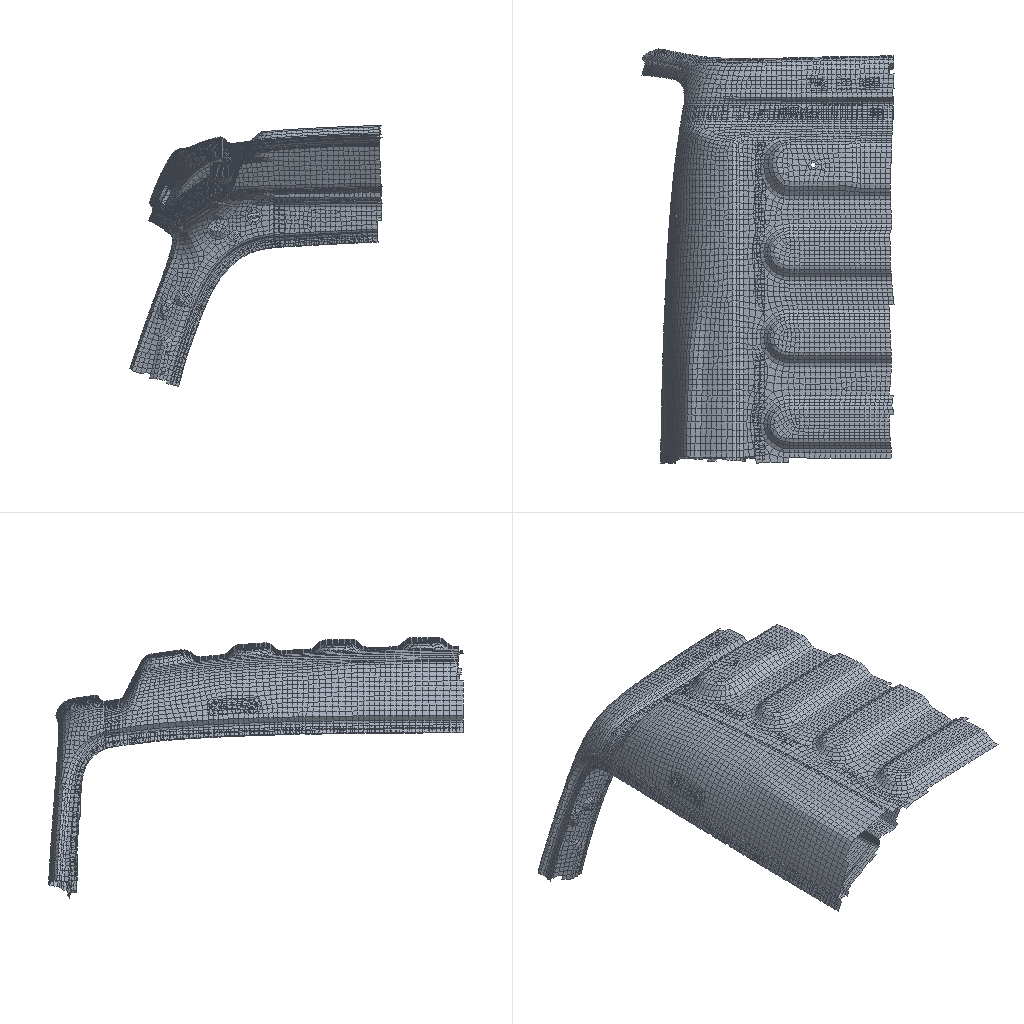Simulation study | nastran
Set-up summary:
category,name,step,type,value,unit,region
solver,nx_nastran
units,not stated in the deck,,not stated
analysis,deck,,static,static
analysis,solution,,SOL,101
load_step,SUBCASE 5,5,SUBCASE,SPC=7 LOAD=8
load_step,SUBCASE 6,6,SUBCASE,SPC=7 LOAD=9
load_step,SUBCASE 7,7,SUBCASE,SPC=7 LOAD=10
load_step,requested,,,3
mesh,nodes,,,11698
mesh,elements,,,10880
element_type,CHEXA,,unverified,49
element_type,CQUAD4,,shell,10507
element_type,CTRIA3,,shell,373
load,load commands in deck,,count,3
bc,support commands in deck,,count,401
check,setup vs results,,match,"every grid point's frame and coordinates and every element id; grid points of CHEXA, CQUAD4, CTRIA3 elements"
Nastran input file, long lists of numbers shortened:
$$------------------------------------------------------------------------------$
$$                                                                              $
$$ NASTRAN Input Deck Generated by HyperMesh Version  : 9.0b121                 $
$$ Generated using HyperMesh-Nastran Template Version : 9.0b121
$$                                                                              $
$$   Template:  general                                                         $
$$                                                                              $
$$------------------------------------------------------------------------------$
$$------------------------------------------------------------------------------$
$$                      Executive Control Cards                                 $
$$------------------------------------------------------------------------------$
SOL 101
CEND
$$------------------------------------------------------------------------------$
$$                      Case Control Cards                                      $
$$------------------------------------------------------------------------------$
  DISPLACEMENT(PLOT) = ALL
$
$HMNAME LOADSTEP               5"LOADX"
SUBCASE       5
  LABEL= LOADX
  SPC =        7
  LOAD =        8
$
$HMNAME LOADSTEP               6"LOADY"
SUBCASE       6
  LABEL= LOADY
  SPC =        7
  LOAD =        9
$
$HMNAME LOADSTEP               7"LOADZ"
SUBCASE       7
  LABEL= LOADZ
  SPC =        7
  LOAD =       10
$$------------------------------------------------------------------------------$
$$                      Bulk Data Cards                                         $
$$------------------------------------------------------------------------------$
BEGIN BULK
PARAM,POST,-1
$$
$$  GRID Data
$$
GRID           3        -862.084668.42731608.46
GRID           4        -860.106668.45771612.594
$ (11696 more lines like these left out)
$$
$$  SPOINT Data
$$
$$
$$------------------------------------------------------------------------------$
$$             Group Definitions                                                $
$$------------------------------------------------------------------------------$
$$
$$ RBE2 Elements - Multiple dependent nodes
$$
RBE2     103454184122190  123456       3       4       5       6       7+
+              8       9      10      11      12      13      14      15+
+             16      17      18      19      20      21      22      23+
+             24      25      26      27      28      29      30      31+
+             32   55580   55581   55582   55583   55584   55585   55586+
+          55587   55588   55589   55590   55591   55592   55593   55594+
+          55595   55596   55597   55598   55599   55600   55601   55602+
+          55603  656174  656175  656180  656181  656201  656202  656207+
+         656209  688645  688646  688651  688659  688660  688664  688665+
+         689069  689070  689071  689072  689073  689074  689075  689076+
+         689077  689078  689079  689080  689094  689096  689098  689102+
+         689104  689107  6891088412161884121619
$
$HMMOVE 84022691
$        1034541
$
$
$  RBE3 Elements
$
RBE3      328623         3757819  1234560.013486     123  6771220.002882+
+            123  6771390.173186     123  6771400.810446     123  677147
RBE3      328624         3757820  1234560.182808     123  6771470.040959+
+            123  6771400.142085     123  6771410.634148     123  677146
$ (780 more lines like these left out)
$
$HMMOVE 57005012
$         328623THRU      328626  328628THRU      328635  328637THRU      328640
$         329091THRU      329094  329096THRU      329103  329105THRU      329112
$         329114THRU      329121  329123THRU      329126  329145THRU      329148
$         329150THRU      329157  329159THRU      329162  332016THRU      332019
$         332021THRU      332024  332178THRU      332181  332183THRU      332190
$         332192THRU      332199  332201THRU      332208  332210THRU      332213
$         332232THRU      332235  332237THRU      332240  332403THRU      332406
$         332408THRU      332415  332417THRU      332424  332426THRU      332433
$         332435THRU      332442  332444THRU      332451  332453THRU      332460
$         332462THRU      332465  340854THRU      340857  340859THRU      340862
$         341115THRU      341118  341120THRU      341123  341178THRU      341181
$         341183THRU      341190  341192THRU      341199  341201THRU      341208
$         341210THRU      341217  341219THRU      341226  341228THRU      341231
$         341349THRU      341352  341354THRU      341357  341376THRU      341379
$         341381THRU      341388  341390THRU      341397  341399THRU      341402
$         341412THRU      341415  341417THRU      341420  341430THRU      341433
$         341435THRU      341438  343293THRU      343296  343298THRU      343305
$         343307THRU      343314  343316THRU      343323  343325THRU      343332
$         343334THRU      343341  343343THRU      343350  343352THRU      343359
$         343361THRU      343368  343370THRU      343377  343379THRU      343382
$         344139THRU      344142  344144THRU      344151  344153THRU      344160
$         344162THRU      344169  344171THRU      344174
$
$$
$$  CTRIA3 Data
$$
CTRIA3    199367       184121618      16     205
CTRIA3    199376       1     210     223      10
$ (371 more lines like these left out)
$
$HMMOVE 57001010
$         199367  199376  199456  199490  199666  199761  200208  200213  200228
$         200232  200244  200256  200439  200454THRU      200455  200888  200891
$ (66 more lines like these left out)
CQUAD4    199311       18412161884121619       3      16
CQUAD4    199312       1      16       3       4      15
$ (10505 more lines like these left out)
$
$HMMOVE 57001010
$         199311THRU      199332  199338THRU      199366  199368THRU      199375
$         199377THRU      199455  199457THRU      199489  199491THRU      199665
$ (379 more lines like these left out)
CHEXA     328627      10 3757819 3757822 3757821 3757820 3757823 3757826+
+        3757825 3757824
CHEXA     328636      10 3757828 3757831 3757830 3757829 3757832 3757835+
+        3757834 3757833
$ (94 more lines like these left out)
$
$HMMOVE 57005011
$         328627  328636  329095  329104  329113  329122  329149  329158  332020
$         332182  332191  332200  332209  332236  332407  332416  332425  332434
$ (60 more lines like these left out)
PSHELL         2       11.2            1               1
$
$
$
$HMNAME PROP                   1"80" 4
$HWCOLOR PROP                  1       3
PSHELL         1       10.8            1               1
$$
$$  PSOLID Data
$
$HMNAME PROP                  10"spot" 5
$HWCOLOR PROP                 10       3
PSOLID        10       1
$$
$$------------------------------------------------------------------------------$
$$                      Material Definition Cards                               $
$$------------------------------------------------------------------------------$
$$--------------------------------------------------------------
$$ HYPERMESH TAGS
$$--------------------------------------------------------------
$$BEGIN TAGS
$$END TAGS
$$
$$  MAT1 Data
$
$HMNAME MAT                    1"steel" "MAT1"
$HWCOLOR MAT                   1       3
MAT1           1210000.0        0.3     7.90E-09
$$
$$
$$
$$------------------------------------------------------------------------------$
$ (43 more lines like these left out)
SPC            7     874  1234560.0
SPC            7    1041  1234560.0
SPC            7     807  1234560.0
SPC            7    1035  1234560.0
$ (397 more lines like these left out)
$$
$$  FORCE Data
$$
FORCE         1084122190       01.0     0.0     0.0     100.0
FORCE          984122190       01.0     0.0     100.0   0.0
FORCE          884122190       01.0     100.0   0.0     0.0
$HMASSEM 5400200       6 sidebody_R
$HMASSEM_IDS    5400203054004010540020405400801054002010
$HMASSEM 5700100       5 5700100
$HMASSEM_IDS    570010105700201057005010
$
ENDDATA
Results summary:
result,analysis,,,static
result,last_loadstep,,,3
result,primary field,,,displacements
result,max displacement,,,0.03567,model units